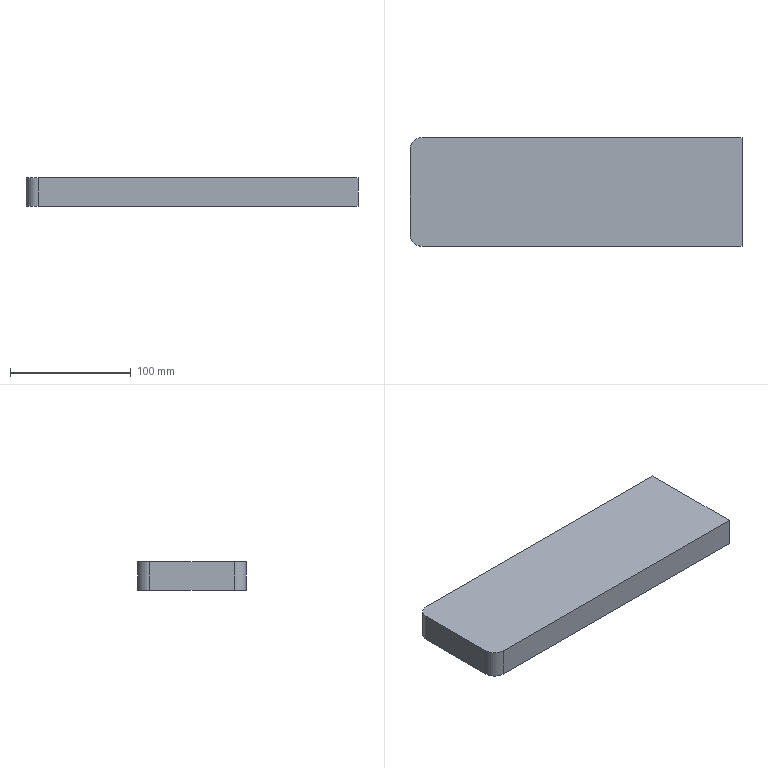Part | SolidWorks | features Extrusion 1 | 1 solid | 8 faces | box 275 x 90 x 23.5 mm | volume 580616 mm3 | plane 6 | cylinder 2 | commonest cylinder face diameters 20 x2
STEP:
#1=CARTESIAN_POINT('',(132.5,-45.,0.));
#2=VERTEX_POINT('',#1);
#3=CARTESIAN_POINT('',(132.5,45.,0.));
#4=VERTEX_POINT('',#3);
#5=CARTESIAN_POINT('',(132.5,-45.,0.));
#6=DIRECTION('',(0.,1.,0.));
#7=VECTOR('',#6,1000.);
#8=LINE('',#5,#7);
#9=EDGE_CURVE('',#2,#4,#8,.T.);
#10=ORIENTED_EDGE('',*,*,#9,.T.);
#11=CARTESIAN_POINT('',(132.5,45.,23.5));
#12=VERTEX_POINT('',#11);
#13=CARTESIAN_POINT('',(132.5,45.,23.5));
#14=DIRECTION('',(0.,0.,-1.));
#15=VECTOR('',#14,1000.);
#16=LINE('',#13,#15);
#17=EDGE_CURVE('',#12,#4,#16,.T.);
#18=ORIENTED_EDGE('',*,*,#17,.F.);
#19=CARTESIAN_POINT('',(132.5,-45.,23.5));
#20=VERTEX_POINT('',#19);
#21=CARTESIAN_POINT('',(132.5,-45.,23.5));
#22=DIRECTION('',(0.,1.,0.));
#23=VECTOR('',#22,1000.);
#24=LINE('',#21,#23);
#25=EDGE_CURVE('',#20,#12,#24,.T.);
#26=ORIENTED_EDGE('',*,*,#25,.F.);
#27=CARTESIAN_POINT('',(132.5,-45.,23.5));
#28=DIRECTION('',(0.,0.,-1.));
#29=VECTOR('',#28,1000.);
#30=LINE('',#27,#29);
#31=EDGE_CURVE('',#20,#2,#30,.T.);
#32=ORIENTED_EDGE('',*,*,#31,.T.);
#33=EDGE_LOOP('',(#10,#18,#26,#32));
#34=FACE_OUTER_BOUND('',#33,.T.);
#35=CARTESIAN_POINT('',(132.5,-45.,23.5));
#36=DIRECTION('',(-1.,0.,0.));
#37=DIRECTION('',(0.,0.,1.));
#38=AXIS2_PLACEMENT_3D('',#35,#36,#37);
#39=PLANE('',#38);
#40=ADVANCED_FACE('',(#34),#39,.F.);
#41=CARTESIAN_POINT('',(-132.5,45.,0.));
#42=VERTEX_POINT('',#41);
#43=CARTESIAN_POINT('',(-132.5,45.,0.));
#44=DIRECTION('',(-1.,0.,0.));
#45=VECTOR('',#44,1000.);
#46=LINE('',#43,#45);
#47=EDGE_CURVE('',#4,#42,#46,.T.);
#48=ORIENTED_EDGE('',*,*,#47,.T.);
#49=CARTESIAN_POINT('',(-132.5,45.,23.5));
#50=VERTEX_POINT('',#49);
#51=CARTESIAN_POINT('',(-132.5,45.,23.5));
#52=DIRECTION('',(0.,0.,-1.));
#53=VECTOR('',#52,1000.);
#54=LINE('',#51,#53);
#55=EDGE_CURVE('',#50,#42,#54,.T.);
#56=ORIENTED_EDGE('',*,*,#55,.F.);
#57=CARTESIAN_POINT('',(-132.5,45.,23.5));
#58=DIRECTION('',(-1.,0.,0.));
#59=VECTOR('',#58,1000.);
#60=LINE('',#57,#59);
#61=EDGE_CURVE('',#12,#50,#60,.T.);
#62=ORIENTED_EDGE('',*,*,#61,.F.);
#63=ORIENTED_EDGE('',*,*,#17,.T.);
#64=EDGE_LOOP('',(#48,#56,#62,#63));
#65=FACE_OUTER_BOUND('',#64,.T.);
#66=CARTESIAN_POINT('',(-132.5,45.,23.5));
#67=DIRECTION('',(0.,-1.,0.));
#68=DIRECTION('',(0.,0.,-1.));
#69=AXIS2_PLACEMENT_3D('',#66,#67,#68);
#70=PLANE('',#69);
#71=ADVANCED_FACE('',(#65),#70,.F.);
#72=CARTESIAN_POINT('',(-142.5,35.,0.));
#73=VERTEX_POINT('',#72);
#74=CARTESIAN_POINT('',(-132.5,35.,0.));
#75=DIRECTION('',(0.,0.,1.));
#76=DIRECTION('',(-1.,0.,0.));
#77=AXIS2_PLACEMENT_3D('',#74,#75,#76);
#78=CIRCLE('',#77,10.);
#79=EDGE_CURVE('',#42,#73,#78,.T.);
#80=ORIENTED_EDGE('',*,*,#79,.T.);
#81=CARTESIAN_POINT('',(-142.5,35.,23.5));
#82=VERTEX_POINT('',#81);
#83=CARTESIAN_POINT('',(-142.5,35.,23.5));
#84=DIRECTION('',(0.,0.,-1.));
#85=VECTOR('',#84,1000.);
#86=LINE('',#83,#85);
#87=EDGE_CURVE('',#82,#73,#86,.T.);
#88=ORIENTED_EDGE('',*,*,#87,.F.);
#89=CARTESIAN_POINT('',(-132.5,35.,23.5));
#90=DIRECTION('',(0.,0.,1.));
#91=DIRECTION('',(-1.,0.,0.));
#92=AXIS2_PLACEMENT_3D('',#89,#90,#91);
#93=CIRCLE('',#92,10.);
#94=EDGE_CURVE('',#50,#82,#93,.T.);
#95=ORIENTED_EDGE('',*,*,#94,.F.);
#96=ORIENTED_EDGE('',*,*,#55,.T.);
#97=EDGE_LOOP('',(#80,#88,#95,#96));
#98=FACE_OUTER_BOUND('',#97,.T.);
#99=CARTESIAN_POINT('',(-132.5,35.,23.5));
#100=DIRECTION('',(0.,0.,-1.));
#101=DIRECTION('',(-1.,0.,0.));
#102=AXIS2_PLACEMENT_3D('',#99,#100,#101);
#103=CYLINDRICAL_SURFACE('',#102,10.);
#104=ADVANCED_FACE('',(#98),#103,.T.);
#105=CARTESIAN_POINT('',(-142.5,-35.,0.));
#106=VERTEX_POINT('',#105);
#107=CARTESIAN_POINT('',(-142.5,-35.,0.));
#108=DIRECTION('',(0.,-1.,0.));
#109=VECTOR('',#108,1000.);
#110=LINE('',#107,#109);
#111=EDGE_CURVE('',#73,#106,#110,.T.);
#112=ORIENTED_EDGE('',*,*,#111,.T.);
#113=CARTESIAN_POINT('',(-142.5,-35.,23.5));
#114=VERTEX_POINT('',#113);
#115=CARTESIAN_POINT('',(-142.5,-35.,23.5));
#116=DIRECTION('',(0.,0.,-1.));
#117=VECTOR('',#116,1000.);
#118=LINE('',#115,#117);
#119=EDGE_CURVE('',#114,#106,#118,.T.);
#120=ORIENTED_EDGE('',*,*,#119,.F.);
#121=CARTESIAN_POINT('',(-142.5,-35.,23.5));
#122=DIRECTION('',(0.,-1.,0.));
#123=VECTOR('',#122,1000.);
#124=LINE('',#121,#123);
#125=EDGE_CURVE('',#82,#114,#124,.T.);
#126=ORIENTED_EDGE('',*,*,#125,.F.);
#127=ORIENTED_EDGE('',*,*,#87,.T.);
#128=EDGE_LOOP('',(#112,#120,#126,#127));
#129=FACE_OUTER_BOUND('',#128,.T.);
#130=CARTESIAN_POINT('',(-142.5,-35.,23.5));
#131=DIRECTION('',(1.,0.,0.));
#132=DIRECTION('',(0.,0.,-1.));
#133=AXIS2_PLACEMENT_3D('',#130,#131,#132);
#134=PLANE('',#133);
#135=ADVANCED_FACE('',(#129),#134,.F.);
#136=CARTESIAN_POINT('',(-132.5,-45.,0.));
#137=VERTEX_POINT('',#136);
#138=CARTESIAN_POINT('',(-132.5,-35.,0.));
#139=DIRECTION('',(0.,0.,1.));
#140=DIRECTION('',(-1.,0.,0.));
#141=AXIS2_PLACEMENT_3D('',#138,#139,#140);
#142=CIRCLE('',#141,10.);
#143=EDGE_CURVE('',#106,#137,#142,.T.);
#144=ORIENTED_EDGE('',*,*,#143,.T.);
#145=CARTESIAN_POINT('',(-132.5,-45.,23.5));
#146=VERTEX_POINT('',#145);
#147=CARTESIAN_POINT('',(-132.5,-45.,23.5));
#148=DIRECTION('',(0.,0.,-1.));
#149=VECTOR('',#148,1000.);
#150=LINE('',#147,#149);
#151=EDGE_CURVE('',#146,#137,#150,.T.);
#152=ORIENTED_EDGE('',*,*,#151,.F.);
#153=CARTESIAN_POINT('',(-132.5,-35.,23.5));
#154=DIRECTION('',(0.,0.,1.));
#155=DIRECTION('',(-1.,0.,0.));
#156=AXIS2_PLACEMENT_3D('',#153,#154,#155);
#157=CIRCLE('',#156,10.);
#158=EDGE_CURVE('',#114,#146,#157,.T.);
#159=ORIENTED_EDGE('',*,*,#158,.F.);
#160=ORIENTED_EDGE('',*,*,#119,.T.);
#161=EDGE_LOOP('',(#144,#152,#159,#160));
#162=FACE_OUTER_BOUND('',#161,.T.);
#163=CARTESIAN_POINT('',(-132.5,-35.,23.5));
#164=DIRECTION('',(0.,0.,-1.));
#165=DIRECTION('',(-1.,0.,0.));
#166=AXIS2_PLACEMENT_3D('',#163,#164,#165);
#167=CYLINDRICAL_SURFACE('',#166,10.);
#168=ADVANCED_FACE('',(#162),#167,.T.);
#169=CARTESIAN_POINT('',(-132.5,-45.,0.));
#170=DIRECTION('',(1.,0.,0.));
#171=VECTOR('',#170,1000.);
#172=LINE('',#169,#171);
#173=EDGE_CURVE('',#137,#2,#172,.T.);
#174=ORIENTED_EDGE('',*,*,#173,.T.);
#175=ORIENTED_EDGE('',*,*,#31,.F.);
#176=CARTESIAN_POINT('',(-132.5,-45.,23.5));
#177=DIRECTION('',(1.,0.,0.));
#178=VECTOR('',#177,1000.);
#179=LINE('',#176,#178);
#180=EDGE_CURVE('',#146,#20,#179,.T.);
#181=ORIENTED_EDGE('',*,*,#180,.F.);
#182=ORIENTED_EDGE('',*,*,#151,.T.);
#183=EDGE_LOOP('',(#174,#175,#181,#182));
#184=FACE_OUTER_BOUND('',#183,.T.);
#185=CARTESIAN_POINT('',(-132.5,-45.,23.5));
#186=DIRECTION('',(0.,1.,0.));
#187=DIRECTION('',(0.,0.,1.));
#188=AXIS2_PLACEMENT_3D('',#185,#186,#187);
#189=PLANE('',#188);
#190=ADVANCED_FACE('',(#184),#189,.F.);
#191=ORIENTED_EDGE('',*,*,#25,.T.);
#192=ORIENTED_EDGE('',*,*,#61,.T.);
#193=ORIENTED_EDGE('',*,*,#94,.T.);
#194=ORIENTED_EDGE('',*,*,#125,.T.);
#195=ORIENTED_EDGE('',*,*,#158,.T.);
#196=ORIENTED_EDGE('',*,*,#180,.T.);
#197=EDGE_LOOP('',(#191,#192,#193,#194,#195,#196));
#198=FACE_OUTER_BOUND('',#197,.T.);
#199=CARTESIAN_POINT('',(-132.5,35.,23.5));
#200=DIRECTION('',(0.,0.,-1.));
#201=DIRECTION('',(-1.,0.,0.));
#202=AXIS2_PLACEMENT_3D('',#199,#200,#201);
#203=PLANE('',#202);
#204=ADVANCED_FACE('',(#198),#203,.F.);
#205=ORIENTED_EDGE('',*,*,#9,.F.);
#206=ORIENTED_EDGE('',*,*,#173,.F.);
#207=ORIENTED_EDGE('',*,*,#143,.F.);
#208=ORIENTED_EDGE('',*,*,#111,.F.);
#209=ORIENTED_EDGE('',*,*,#79,.F.);
#210=ORIENTED_EDGE('',*,*,#47,.F.);
#211=EDGE_LOOP('',(#205,#206,#207,#208,#209,#210));
#212=FACE_OUTER_BOUND('',#211,.T.);
#213=CARTESIAN_POINT('',(-132.5,35.,0.));
#214=DIRECTION('',(0.,0.,-1.));
#215=DIRECTION('',(-1.,0.,0.));
#216=AXIS2_PLACEMENT_3D('',#213,#214,#215);
#217=PLANE('',#216);
#218=ADVANCED_FACE('',(#212),#217,.T.);
#219=CLOSED_SHELL('',(#40,#71,#104,#135,#168,#190,#204,#218));
#220=MANIFOLD_SOLID_BREP('',#219);
#221=CARTESIAN_POINT('',(0.,0.,0.));
#222=DIRECTION('',(0.,0.,1.));
#223=DIRECTION('',(1.,0.,0.));
#224=AXIS2_PLACEMENT_3D('',#221,#222,#223);
#225=(LENGTH_UNIT()NAMED_UNIT(*)SI_UNIT(.MILLI.,.METRE.));
#226=UNCERTAINTY_MEASURE_WITH_UNIT(LENGTH_MEASURE(0.00001),#225,'','');
#227=(NAMED_UNIT(*)PLANE_ANGLE_UNIT()SI_UNIT($,.RADIAN.));
#228=(NAMED_UNIT(*)SI_UNIT($,.STERADIAN.)SOLID_ANGLE_UNIT());
#229=(GEOMETRIC_REPRESENTATION_CONTEXT(3)GLOBAL_UNCERTAINTY_ASSIGNED_CONTEXT((#226))GLOBAL_UNIT_ASSIGNED_CONTEXT((#225,#227,#228))REPRESENTATION_CONTEXT('',''));
#230=ADVANCED_BREP_SHAPE_REPRESENTATION('',(#220,#224),#229);